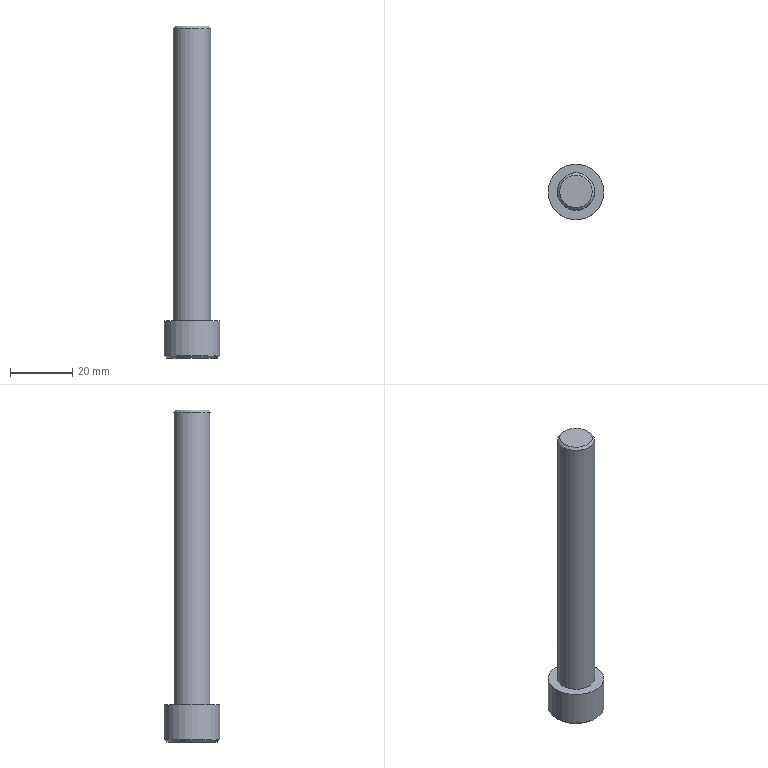Part | STEP file | M12.00-95.00 | 1 solid | 14 faces | box 18 x 18 x 107 mm | volume 13199 mm3 | plane 10 | cylinder 2 | cone 2 | commonest cylinder face diameters 12 x1 18 x1